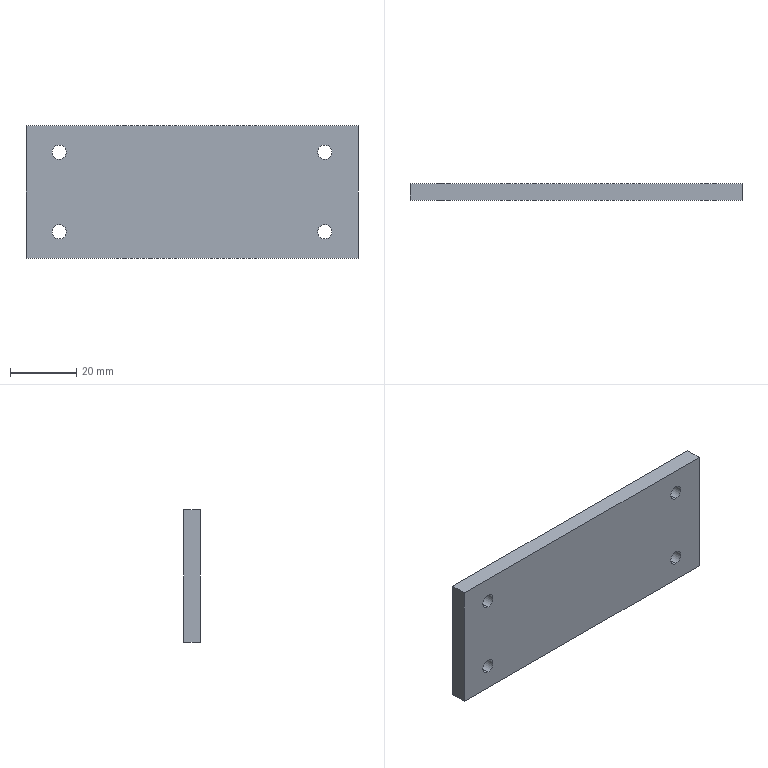Part | SolidWorks | features BaseBody 1 | 1 solid | 14 faces | box 100 x 5 x 40 mm | volume 19710 mm3 | cylinder 8 | plane 6 | commonest cylinder face diameters 4.3 x8
STEP:
#1=CARTESIAN_POINT('',(40.,-2.5,14.15));
#2=VERTEX_POINT('',#1);
#3=CARTESIAN_POINT('',(40.,-2.5,9.85));
#4=VERTEX_POINT('',#3);
#5=CARTESIAN_POINT('',(40.,-2.5,12.));
#6=DIRECTION('',(0.,-1.,0.));
#7=DIRECTION('',(0.,0.,1.));
#8=AXIS2_PLACEMENT_3D('',#5,#6,#7);
#9=CIRCLE('',#8,2.15);
#10=EDGE_CURVE('',#2,#4,#9,.T.);
#11=ORIENTED_EDGE('',*,*,#10,.T.);
#12=CARTESIAN_POINT('',(40.,2.5,9.85));
#13=VERTEX_POINT('',#12);
#14=CARTESIAN_POINT('',(40.,-9.7,9.85));
#15=DIRECTION('',(0.,1.,0.));
#16=VECTOR('',#15,1000.);
#17=LINE('',#14,#16);
#18=EDGE_CURVE('',#4,#13,#17,.T.);
#19=ORIENTED_EDGE('',*,*,#18,.T.);
#20=CARTESIAN_POINT('',(40.,2.5,14.15));
#21=VERTEX_POINT('',#20);
#22=CARTESIAN_POINT('',(40.,2.5,12.));
#23=DIRECTION('',(0.,-1.,0.));
#24=DIRECTION('',(0.,0.,1.));
#25=AXIS2_PLACEMENT_3D('',#22,#23,#24);
#26=CIRCLE('',#25,2.15);
#27=EDGE_CURVE('',#21,#13,#26,.T.);
#28=ORIENTED_EDGE('',*,*,#27,.F.);
#29=CARTESIAN_POINT('',(40.,-9.7,14.15));
#30=DIRECTION('',(0.,1.,0.));
#31=VECTOR('',#30,1000.);
#32=LINE('',#29,#31);
#33=EDGE_CURVE('',#2,#21,#32,.T.);
#34=ORIENTED_EDGE('',*,*,#33,.F.);
#35=EDGE_LOOP('',(#11,#19,#28,#34));
#36=FACE_OUTER_BOUND('',#35,.T.);
#37=CARTESIAN_POINT('',(40.,-9.7,12.));
#38=DIRECTION('',(0.,1.,0.));
#39=DIRECTION('',(0.,0.,1.));
#40=AXIS2_PLACEMENT_3D('',#37,#38,#39);
#41=CYLINDRICAL_SURFACE('',#40,2.15);
#42=ADVANCED_FACE('',(#36),#41,.F.);
#43=CARTESIAN_POINT('',(40.,-2.5,-9.85));
#44=VERTEX_POINT('',#43);
#45=CARTESIAN_POINT('',(40.,-2.5,-14.15));
#46=VERTEX_POINT('',#45);
#47=CARTESIAN_POINT('',(40.,-2.5,-12.));
#48=DIRECTION('',(0.,-1.,0.));
#49=DIRECTION('',(0.,0.,1.));
#50=AXIS2_PLACEMENT_3D('',#47,#48,#49);
#51=CIRCLE('',#50,2.15);
#52=EDGE_CURVE('',#44,#46,#51,.T.);
#53=ORIENTED_EDGE('',*,*,#52,.T.);
#54=CARTESIAN_POINT('',(40.,2.5,-14.15));
#55=VERTEX_POINT('',#54);
#56=CARTESIAN_POINT('',(40.,-9.7,-14.15));
#57=DIRECTION('',(0.,1.,0.));
#58=VECTOR('',#57,1000.);
#59=LINE('',#56,#58);
#60=EDGE_CURVE('',#46,#55,#59,.T.);
#61=ORIENTED_EDGE('',*,*,#60,.T.);
#62=CARTESIAN_POINT('',(40.,2.5,-9.85));
#63=VERTEX_POINT('',#62);
#64=CARTESIAN_POINT('',(40.,2.5,-12.));
#65=DIRECTION('',(0.,-1.,0.));
#66=DIRECTION('',(0.,0.,1.));
#67=AXIS2_PLACEMENT_3D('',#64,#65,#66);
#68=CIRCLE('',#67,2.15);
#69=EDGE_CURVE('',#63,#55,#68,.T.);
#70=ORIENTED_EDGE('',*,*,#69,.F.);
#71=CARTESIAN_POINT('',(40.,-9.7,-9.85));
#72=DIRECTION('',(0.,1.,0.));
#73=VECTOR('',#72,1000.);
#74=LINE('',#71,#73);
#75=EDGE_CURVE('',#44,#63,#74,.T.);
#76=ORIENTED_EDGE('',*,*,#75,.F.);
#77=EDGE_LOOP('',(#53,#61,#70,#76));
#78=FACE_OUTER_BOUND('',#77,.T.);
#79=CARTESIAN_POINT('',(40.,-9.7,-12.));
#80=DIRECTION('',(0.,1.,0.));
#81=DIRECTION('',(0.,0.,1.));
#82=AXIS2_PLACEMENT_3D('',#79,#80,#81);
#83=CYLINDRICAL_SURFACE('',#82,2.15);
#84=ADVANCED_FACE('',(#78),#83,.F.);
#85=CARTESIAN_POINT('',(-40.,-2.5,14.15));
#86=VERTEX_POINT('',#85);
#87=CARTESIAN_POINT('',(-40.,-2.5,9.85));
#88=VERTEX_POINT('',#87);
#89=CARTESIAN_POINT('',(-40.,-2.5,12.));
#90=DIRECTION('',(0.,-1.,0.));
#91=DIRECTION('',(0.,0.,1.));
#92=AXIS2_PLACEMENT_3D('',#89,#90,#91);
#93=CIRCLE('',#92,2.15);
#94=EDGE_CURVE('',#86,#88,#93,.T.);
#95=ORIENTED_EDGE('',*,*,#94,.T.);
#96=CARTESIAN_POINT('',(-40.,2.5,9.85));
#97=VERTEX_POINT('',#96);
#98=CARTESIAN_POINT('',(-40.,-9.7,9.85));
#99=DIRECTION('',(0.,1.,0.));
#100=VECTOR('',#99,1000.);
#101=LINE('',#98,#100);
#102=EDGE_CURVE('',#88,#97,#101,.T.);
#103=ORIENTED_EDGE('',*,*,#102,.T.);
#104=CARTESIAN_POINT('',(-40.,2.5,14.15));
#105=VERTEX_POINT('',#104);
#106=CARTESIAN_POINT('',(-40.,2.5,12.));
#107=DIRECTION('',(0.,-1.,0.));
#108=DIRECTION('',(0.,0.,1.));
#109=AXIS2_PLACEMENT_3D('',#106,#107,#108);
#110=CIRCLE('',#109,2.15);
#111=EDGE_CURVE('',#105,#97,#110,.T.);
#112=ORIENTED_EDGE('',*,*,#111,.F.);
#113=CARTESIAN_POINT('',(-40.,-9.7,14.15));
#114=DIRECTION('',(0.,1.,0.));
#115=VECTOR('',#114,1000.);
#116=LINE('',#113,#115);
#117=EDGE_CURVE('',#86,#105,#116,.T.);
#118=ORIENTED_EDGE('',*,*,#117,.F.);
#119=EDGE_LOOP('',(#95,#103,#112,#118));
#120=FACE_OUTER_BOUND('',#119,.T.);
#121=CARTESIAN_POINT('',(-40.,-9.7,12.));
#122=DIRECTION('',(0.,1.,0.));
#123=DIRECTION('',(0.,0.,1.));
#124=AXIS2_PLACEMENT_3D('',#121,#122,#123);
#125=CYLINDRICAL_SURFACE('',#124,2.15);
#126=ADVANCED_FACE('',(#120),#125,.F.);
#127=CARTESIAN_POINT('',(-40.,-2.5,-9.85));
#128=VERTEX_POINT('',#127);
#129=CARTESIAN_POINT('',(-40.,-2.5,-14.15));
#130=VERTEX_POINT('',#129);
#131=CARTESIAN_POINT('',(-40.,-2.5,-12.));
#132=DIRECTION('',(0.,-1.,0.));
#133=DIRECTION('',(0.,0.,1.));
#134=AXIS2_PLACEMENT_3D('',#131,#132,#133);
#135=CIRCLE('',#134,2.15);
#136=EDGE_CURVE('',#128,#130,#135,.T.);
#137=ORIENTED_EDGE('',*,*,#136,.T.);
#138=CARTESIAN_POINT('',(-40.,2.5,-14.15));
#139=VERTEX_POINT('',#138);
#140=CARTESIAN_POINT('',(-40.,-9.7,-14.15));
#141=DIRECTION('',(0.,1.,0.));
#142=VECTOR('',#141,1000.);
#143=LINE('',#140,#142);
#144=EDGE_CURVE('',#130,#139,#143,.T.);
#145=ORIENTED_EDGE('',*,*,#144,.T.);
#146=CARTESIAN_POINT('',(-40.,2.5,-9.85));
#147=VERTEX_POINT('',#146);
#148=CARTESIAN_POINT('',(-40.,2.5,-12.));
#149=DIRECTION('',(0.,-1.,0.));
#150=DIRECTION('',(0.,0.,1.));
#151=AXIS2_PLACEMENT_3D('',#148,#149,#150);
#152=CIRCLE('',#151,2.15);
#153=EDGE_CURVE('',#147,#139,#152,.T.);
#154=ORIENTED_EDGE('',*,*,#153,.F.);
#155=CARTESIAN_POINT('',(-40.,-9.7,-9.85));
#156=DIRECTION('',(0.,1.,0.));
#157=VECTOR('',#156,1000.);
#158=LINE('',#155,#157);
#159=EDGE_CURVE('',#128,#147,#158,.T.);
#160=ORIENTED_EDGE('',*,*,#159,.F.);
#161=EDGE_LOOP('',(#137,#145,#154,#160));
#162=FACE_OUTER_BOUND('',#161,.T.);
#163=CARTESIAN_POINT('',(-40.,-9.7,-12.));
#164=DIRECTION('',(0.,1.,0.));
#165=DIRECTION('',(0.,0.,1.));
#166=AXIS2_PLACEMENT_3D('',#163,#164,#165);
#167=CYLINDRICAL_SURFACE('',#166,2.15);
#168=ADVANCED_FACE('',(#162),#167,.F.);
#169=ORIENTED_EDGE('',*,*,#10,.F.);
#170=CARTESIAN_POINT('',(40.,-2.5,12.));
#171=DIRECTION('',(0.,-1.,0.));
#172=DIRECTION('',(0.,0.,1.));
#173=AXIS2_PLACEMENT_3D('',#170,#171,#172);
#174=CIRCLE('',#173,2.15);
#175=EDGE_CURVE('',#4,#2,#174,.T.);
#176=ORIENTED_EDGE('',*,*,#175,.F.);
#177=EDGE_LOOP('',(#169,#176));
#178=FACE_BOUND('',#177,.T.);
#179=ORIENTED_EDGE('',*,*,#52,.F.);
#180=CARTESIAN_POINT('',(40.,-2.5,-12.));
#181=DIRECTION('',(0.,-1.,0.));
#182=DIRECTION('',(0.,0.,1.));
#183=AXIS2_PLACEMENT_3D('',#180,#181,#182);
#184=CIRCLE('',#183,2.15);
#185=EDGE_CURVE('',#46,#44,#184,.T.);
#186=ORIENTED_EDGE('',*,*,#185,.F.);
#187=EDGE_LOOP('',(#179,#186));
#188=FACE_BOUND('',#187,.T.);
#189=ORIENTED_EDGE('',*,*,#94,.F.);
#190=CARTESIAN_POINT('',(-40.,-2.5,12.));
#191=DIRECTION('',(0.,-1.,0.));
#192=DIRECTION('',(0.,0.,1.));
#193=AXIS2_PLACEMENT_3D('',#190,#191,#192);
#194=CIRCLE('',#193,2.15);
#195=EDGE_CURVE('',#88,#86,#194,.T.);
#196=ORIENTED_EDGE('',*,*,#195,.F.);
#197=EDGE_LOOP('',(#189,#196));
#198=FACE_BOUND('',#197,.T.);
#199=ORIENTED_EDGE('',*,*,#136,.F.);
#200=CARTESIAN_POINT('',(-40.,-2.5,-12.));
#201=DIRECTION('',(0.,-1.,0.));
#202=DIRECTION('',(0.,0.,1.));
#203=AXIS2_PLACEMENT_3D('',#200,#201,#202);
#204=CIRCLE('',#203,2.15);
#205=EDGE_CURVE('',#130,#128,#204,.T.);
#206=ORIENTED_EDGE('',*,*,#205,.F.);
#207=EDGE_LOOP('',(#199,#206));
#208=FACE_BOUND('',#207,.T.);
#209=CARTESIAN_POINT('',(-50.,-2.5,20.));
#210=VERTEX_POINT('',#209);
#211=CARTESIAN_POINT('',(50.,-2.5,20.));
#212=VERTEX_POINT('',#211);
#213=CARTESIAN_POINT('',(-50.,-2.5,20.));
#214=DIRECTION('',(1.,0.,0.));
#215=VECTOR('',#214,1000.);
#216=LINE('',#213,#215);
#217=EDGE_CURVE('',#210,#212,#216,.T.);
#218=ORIENTED_EDGE('',*,*,#217,.F.);
#219=CARTESIAN_POINT('',(-50.,-2.5,-20.));
#220=VERTEX_POINT('',#219);
#221=CARTESIAN_POINT('',(-50.,-2.5,-20.));
#222=DIRECTION('',(0.,0.,1.));
#223=VECTOR('',#222,1000.);
#224=LINE('',#221,#223);
#225=EDGE_CURVE('',#220,#210,#224,.T.);
#226=ORIENTED_EDGE('',*,*,#225,.F.);
#227=CARTESIAN_POINT('',(50.,-2.5,-20.));
#228=VERTEX_POINT('',#227);
#229=CARTESIAN_POINT('',(-50.,-2.5,-20.));
#230=DIRECTION('',(-1.,0.,0.));
#231=VECTOR('',#230,1000.);
#232=LINE('',#229,#231);
#233=EDGE_CURVE('',#228,#220,#232,.T.);
#234=ORIENTED_EDGE('',*,*,#233,.F.);
#235=CARTESIAN_POINT('',(50.,-2.5,-20.));
#236=DIRECTION('',(0.,0.,-1.));
#237=VECTOR('',#236,1000.);
#238=LINE('',#235,#237);
#239=EDGE_CURVE('',#212,#228,#238,.T.);
#240=ORIENTED_EDGE('',*,*,#239,.F.);
#241=EDGE_LOOP('',(#218,#226,#234,#240));
#242=FACE_OUTER_BOUND('',#241,.T.);
#243=CARTESIAN_POINT('',(-50.,-2.5,-20.));
#244=DIRECTION('',(0.,1.,0.));
#245=DIRECTION('',(0.,0.,1.));
#246=AXIS2_PLACEMENT_3D('',#243,#244,#245);
#247=PLANE('',#246);
#248=ADVANCED_FACE('',(#178,#188,#198,#208,#242),#247,.F.);
#249=ORIENTED_EDGE('',*,*,#18,.F.);
#250=ORIENTED_EDGE('',*,*,#175,.T.);
#251=ORIENTED_EDGE('',*,*,#33,.T.);
#252=CARTESIAN_POINT('',(40.,2.5,12.));
#253=DIRECTION('',(0.,-1.,0.));
#254=DIRECTION('',(0.,0.,1.));
#255=AXIS2_PLACEMENT_3D('',#252,#253,#254);
#256=CIRCLE('',#255,2.15);
#257=EDGE_CURVE('',#13,#21,#256,.T.);
#258=ORIENTED_EDGE('',*,*,#257,.F.);
#259=EDGE_LOOP('',(#249,#250,#251,#258));
#260=FACE_OUTER_BOUND('',#259,.T.);
#261=CARTESIAN_POINT('',(40.,-9.7,12.));
#262=DIRECTION('',(0.,1.,0.));
#263=DIRECTION('',(0.,0.,1.));
#264=AXIS2_PLACEMENT_3D('',#261,#262,#263);
#265=CYLINDRICAL_SURFACE('',#264,2.15);
#266=ADVANCED_FACE('',(#260),#265,.F.);
#267=ORIENTED_EDGE('',*,*,#60,.F.);
#268=ORIENTED_EDGE('',*,*,#185,.T.);
#269=ORIENTED_EDGE('',*,*,#75,.T.);
#270=CARTESIAN_POINT('',(40.,2.5,-12.));
#271=DIRECTION('',(0.,-1.,0.));
#272=DIRECTION('',(0.,0.,1.));
#273=AXIS2_PLACEMENT_3D('',#270,#271,#272);
#274=CIRCLE('',#273,2.15);
#275=EDGE_CURVE('',#55,#63,#274,.T.);
#276=ORIENTED_EDGE('',*,*,#275,.F.);
#277=EDGE_LOOP('',(#267,#268,#269,#276));
#278=FACE_OUTER_BOUND('',#277,.T.);
#279=CARTESIAN_POINT('',(40.,-9.7,-12.));
#280=DIRECTION('',(0.,1.,0.));
#281=DIRECTION('',(0.,0.,1.));
#282=AXIS2_PLACEMENT_3D('',#279,#280,#281);
#283=CYLINDRICAL_SURFACE('',#282,2.15);
#284=ADVANCED_FACE('',(#278),#283,.F.);
#285=ORIENTED_EDGE('',*,*,#102,.F.);
#286=ORIENTED_EDGE('',*,*,#195,.T.);
#287=ORIENTED_EDGE('',*,*,#117,.T.);
#288=CARTESIAN_POINT('',(-40.,2.5,12.));
#289=DIRECTION('',(0.,-1.,0.));
#290=DIRECTION('',(0.,0.,1.));
#291=AXIS2_PLACEMENT_3D('',#288,#289,#290);
#292=CIRCLE('',#291,2.15);
#293=EDGE_CURVE('',#97,#105,#292,.T.);
#294=ORIENTED_EDGE('',*,*,#293,.F.);
#295=EDGE_LOOP('',(#285,#286,#287,#294));
#296=FACE_OUTER_BOUND('',#295,.T.);
#297=CARTESIAN_POINT('',(-40.,-9.7,12.));
#298=DIRECTION('',(0.,1.,0.));
#299=DIRECTION('',(0.,0.,1.));
#300=AXIS2_PLACEMENT_3D('',#297,#298,#299);
#301=CYLINDRICAL_SURFACE('',#300,2.15);
#302=ADVANCED_FACE('',(#296),#301,.F.);
#303=ORIENTED_EDGE('',*,*,#144,.F.);
#304=ORIENTED_EDGE('',*,*,#205,.T.);
#305=ORIENTED_EDGE('',*,*,#159,.T.);
#306=CARTESIAN_POINT('',(-40.,2.5,-12.));
#307=DIRECTION('',(0.,-1.,0.));
#308=DIRECTION('',(0.,0.,1.));
#309=AXIS2_PLACEMENT_3D('',#306,#307,#308);
#310=CIRCLE('',#309,2.15);
#311=EDGE_CURVE('',#139,#147,#310,.T.);
#312=ORIENTED_EDGE('',*,*,#311,.F.);
#313=EDGE_LOOP('',(#303,#304,#305,#312));
#314=FACE_OUTER_BOUND('',#313,.T.);
#315=CARTESIAN_POINT('',(-40.,-9.7,-12.));
#316=DIRECTION('',(0.,1.,0.));
#317=DIRECTION('',(0.,0.,1.));
#318=AXIS2_PLACEMENT_3D('',#315,#316,#317);
#319=CYLINDRICAL_SURFACE('',#318,2.15);
#320=ADVANCED_FACE('',(#314),#319,.F.);
#321=CARTESIAN_POINT('',(50.,2.5,-20.));
#322=VERTEX_POINT('',#321);
#323=CARTESIAN_POINT('',(50.,2.5,20.));
#324=VERTEX_POINT('',#323);
#325=CARTESIAN_POINT('',(50.,2.5,-20.));
#326=DIRECTION('',(0.,0.,1.));
#327=VECTOR('',#326,1000.);
#328=LINE('',#325,#327);
#329=EDGE_CURVE('',#322,#324,#328,.T.);
#330=ORIENTED_EDGE('',*,*,#329,.T.);
#331=CARTESIAN_POINT('',(50.,-2.5,20.));
#332=DIRECTION('',(0.,-1.,0.));
#333=VECTOR('',#332,1000.);
#334=LINE('',#331,#333);
#335=EDGE_CURVE('',#324,#212,#334,.T.);
#336=ORIENTED_EDGE('',*,*,#335,.T.);
#337=ORIENTED_EDGE('',*,*,#239,.T.);
#338=CARTESIAN_POINT('',(50.,-2.5,-20.));
#339=DIRECTION('',(0.,1.,0.));
#340=VECTOR('',#339,1000.);
#341=LINE('',#338,#340);
#342=EDGE_CURVE('',#228,#322,#341,.T.);
#343=ORIENTED_EDGE('',*,*,#342,.T.);
#344=EDGE_LOOP('',(#330,#336,#337,#343));
#345=FACE_OUTER_BOUND('',#344,.T.);
#346=CARTESIAN_POINT('',(50.,-2.5,-20.));
#347=DIRECTION('',(1.,0.,0.));
#348=DIRECTION('',(0.,0.,-1.));
#349=AXIS2_PLACEMENT_3D('',#346,#347,#348);
#350=PLANE('',#349);
#351=ADVANCED_FACE('',(#345),#350,.T.);
#352=ORIENTED_EDGE('',*,*,#335,.F.);
#353=CARTESIAN_POINT('',(-50.,2.5,20.));
#354=VERTEX_POINT('',#353);
#355=CARTESIAN_POINT('',(-50.,2.5,20.));
#356=DIRECTION('',(-1.,0.,0.));
#357=VECTOR('',#356,1000.);
#358=LINE('',#355,#357);
#359=EDGE_CURVE('',#324,#354,#358,.T.);
#360=ORIENTED_EDGE('',*,*,#359,.T.);
#361=CARTESIAN_POINT('',(-50.,-2.5,20.));
#362=DIRECTION('',(0.,-1.,0.));
#363=VECTOR('',#362,1000.);
#364=LINE('',#361,#363);
#365=EDGE_CURVE('',#354,#210,#364,.T.);
#366=ORIENTED_EDGE('',*,*,#365,.T.);
#367=ORIENTED_EDGE('',*,*,#217,.T.);
#368=EDGE_LOOP('',(#352,#360,#366,#367));
#369=FACE_OUTER_BOUND('',#368,.T.);
#370=CARTESIAN_POINT('',(-50.,-2.5,20.));
#371=DIRECTION('',(0.,0.,1.));
#372=DIRECTION('',(1.,0.,0.));
#373=AXIS2_PLACEMENT_3D('',#370,#371,#372);
#374=PLANE('',#373);
#375=ADVANCED_FACE('',(#369),#374,.T.);
#376=CARTESIAN_POINT('',(-50.,2.5,-20.));
#377=VERTEX_POINT('',#376);
#378=CARTESIAN_POINT('',(-50.,2.5,-20.));
#379=DIRECTION('',(0.,0.,1.));
#380=VECTOR('',#379,1000.);
#381=LINE('',#378,#380);
#382=EDGE_CURVE('',#377,#354,#381,.T.);
#383=ORIENTED_EDGE('',*,*,#382,.F.);
#384=CARTESIAN_POINT('',(-50.,-2.5,-20.));
#385=DIRECTION('',(0.,1.,0.));
#386=VECTOR('',#385,1000.);
#387=LINE('',#384,#386);
#388=EDGE_CURVE('',#220,#377,#387,.T.);
#389=ORIENTED_EDGE('',*,*,#388,.F.);
#390=ORIENTED_EDGE('',*,*,#225,.T.);
#391=ORIENTED_EDGE('',*,*,#365,.F.);
#392=EDGE_LOOP('',(#383,#389,#390,#391));
#393=FACE_OUTER_BOUND('',#392,.T.);
#394=CARTESIAN_POINT('',(-50.,-2.5,-20.));
#395=DIRECTION('',(1.,0.,0.));
#396=DIRECTION('',(0.,0.,-1.));
#397=AXIS2_PLACEMENT_3D('',#394,#395,#396);
#398=PLANE('',#397);
#399=ADVANCED_FACE('',(#393),#398,.F.);
#400=ORIENTED_EDGE('',*,*,#342,.F.);
#401=ORIENTED_EDGE('',*,*,#233,.T.);
#402=ORIENTED_EDGE('',*,*,#388,.T.);
#403=CARTESIAN_POINT('',(-50.,2.5,-20.));
#404=DIRECTION('',(-1.,0.,0.));
#405=VECTOR('',#404,1000.);
#406=LINE('',#403,#405);
#407=EDGE_CURVE('',#322,#377,#406,.T.);
#408=ORIENTED_EDGE('',*,*,#407,.F.);
#409=EDGE_LOOP('',(#400,#401,#402,#408));
#410=FACE_OUTER_BOUND('',#409,.T.);
#411=CARTESIAN_POINT('',(-50.,-2.5,-20.));
#412=DIRECTION('',(0.,0.,1.));
#413=DIRECTION('',(1.,0.,0.));
#414=AXIS2_PLACEMENT_3D('',#411,#412,#413);
#415=PLANE('',#414);
#416=ADVANCED_FACE('',(#410),#415,.F.);
#417=ORIENTED_EDGE('',*,*,#27,.T.);
#418=ORIENTED_EDGE('',*,*,#257,.T.);
#419=EDGE_LOOP('',(#417,#418));
#420=FACE_BOUND('',#419,.T.);
#421=ORIENTED_EDGE('',*,*,#69,.T.);
#422=ORIENTED_EDGE('',*,*,#275,.T.);
#423=EDGE_LOOP('',(#421,#422));
#424=FACE_BOUND('',#423,.T.);
#425=ORIENTED_EDGE('',*,*,#111,.T.);
#426=ORIENTED_EDGE('',*,*,#293,.T.);
#427=EDGE_LOOP('',(#425,#426));
#428=FACE_BOUND('',#427,.T.);
#429=ORIENTED_EDGE('',*,*,#153,.T.);
#430=ORIENTED_EDGE('',*,*,#311,.T.);
#431=EDGE_LOOP('',(#429,#430));
#432=FACE_BOUND('',#431,.T.);
#433=ORIENTED_EDGE('',*,*,#359,.F.);
#434=ORIENTED_EDGE('',*,*,#329,.F.);
#435=ORIENTED_EDGE('',*,*,#407,.T.);
#436=ORIENTED_EDGE('',*,*,#382,.T.);
#437=EDGE_LOOP('',(#433,#434,#435,#436));
#438=FACE_OUTER_BOUND('',#437,.T.);
#439=CARTESIAN_POINT('',(-50.,2.5,-20.));
#440=DIRECTION('',(0.,1.,0.));
#441=DIRECTION('',(0.,0.,1.));
#442=AXIS2_PLACEMENT_3D('',#439,#440,#441);
#443=PLANE('',#442);
#444=ADVANCED_FACE('',(#420,#424,#428,#432,#438),#443,.T.);
#445=CLOSED_SHELL('',(#42,#84,#126,#168,#248,#266,#284,#302,#320,#351,#375,#399,#416,#444));
#446=MANIFOLD_SOLID_BREP('',#445);
#447=CARTESIAN_POINT('',(0.,0.,0.));
#448=DIRECTION('',(0.,0.,1.));
#449=DIRECTION('',(1.,0.,0.));
#450=AXIS2_PLACEMENT_3D('',#447,#448,#449);
#451=(LENGTH_UNIT()NAMED_UNIT(*)SI_UNIT(.MILLI.,.METRE.));
#452=UNCERTAINTY_MEASURE_WITH_UNIT(LENGTH_MEASURE(0.00001),#451,'','');
#453=(NAMED_UNIT(*)PLANE_ANGLE_UNIT()SI_UNIT($,.RADIAN.));
#454=(NAMED_UNIT(*)SI_UNIT($,.STERADIAN.)SOLID_ANGLE_UNIT());
#455=(GEOMETRIC_REPRESENTATION_CONTEXT(3)GLOBAL_UNCERTAINTY_ASSIGNED_CONTEXT((#452))GLOBAL_UNIT_ASSIGNED_CONTEXT((#451,#453,#454))REPRESENTATION_CONTEXT('',''));
#456=ADVANCED_BREP_SHAPE_REPRESENTATION('',(#446,#450),#455);